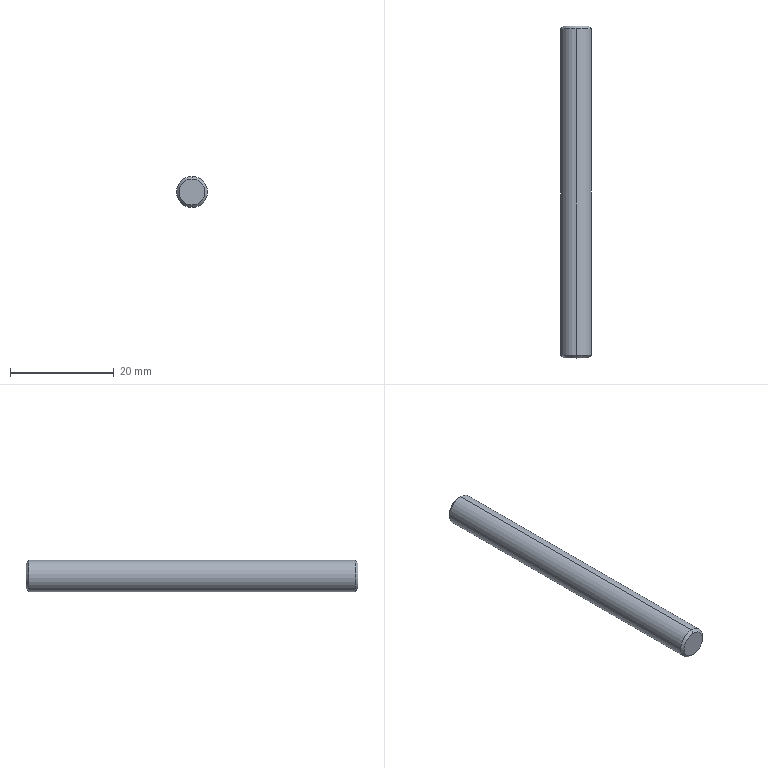Part | NX | features BREP 1 | 1 solid | 8 faces | box 6 x 64 x 6 mm | volume 1805 mm3 | cone 4 | cylinder 2 | plane 2 | commonest cylinder face diameters 6 x2
STEP:
#1=CARTESIAN_POINT('',(0.,64.,2.5));
#2=VERTEX_POINT('',#1);
#3=CARTESIAN_POINT('',(0.,64.,-2.5));
#4=VERTEX_POINT('',#3);
#5=CARTESIAN_POINT('',(0.,64.,0.));
#6=DIRECTION('',(0.,1.,0.));
#7=DIRECTION('',(0.,0.,1.));
#8=AXIS2_PLACEMENT_3D('',#5,#6,#7);
#9=CIRCLE('',#8,2.5);
#10=EDGE_CURVE('',#2,#4,#9,.T.);
#11=ORIENTED_EDGE('',*,*,#10,.F.);
#12=CARTESIAN_POINT('',(0.,63.5,3.));
#13=VERTEX_POINT('',#12);
#14=CARTESIAN_POINT('',(0.,64.,2.5));
#15=DIRECTION('',(0.,-0.7071,0.7071));
#16=VECTOR('',#15,1000.);
#17=LINE('',#14,#16);
#18=EDGE_CURVE('',#13,#2,#17,.F.);
#19=ORIENTED_EDGE('',*,*,#18,.F.);
#20=CARTESIAN_POINT('',(0.,63.5,-3.));
#21=VERTEX_POINT('',#20);
#22=CARTESIAN_POINT('',(0.,63.5,0.));
#23=DIRECTION('',(0.,-1.,0.));
#24=DIRECTION('',(0.,0.,1.));
#25=AXIS2_PLACEMENT_3D('',#22,#23,#24);
#26=CIRCLE('',#25,3.);
#27=EDGE_CURVE('',#21,#13,#26,.T.);
#28=ORIENTED_EDGE('',*,*,#27,.F.);
#29=CARTESIAN_POINT('',(0.,64.,-2.5));
#30=DIRECTION('',(0.,-0.7071,-0.7071));
#31=VECTOR('',#30,1000.);
#32=LINE('',#29,#31);
#33=EDGE_CURVE('',#21,#4,#32,.F.);
#34=ORIENTED_EDGE('',*,*,#33,.T.);
#35=EDGE_LOOP('',(#11,#19,#28,#34));
#36=FACE_BOUND('',#35,.T.);
#37=CARTESIAN_POINT('',(0.,64.,0.));
#38=DIRECTION('',(0.,-1.,0.));
#39=DIRECTION('',(0.,0.,1.));
#40=AXIS2_PLACEMENT_3D('',#37,#38,#39);
#41=CONICAL_SURFACE('',#40,2.5,0.7854);
#42=ADVANCED_FACE('',(#36),#41,.T.);
#43=CARTESIAN_POINT('',(0.,0.,-2.5));
#44=VERTEX_POINT('',#43);
#45=CARTESIAN_POINT('',(0.,0.,2.5));
#46=VERTEX_POINT('',#45);
#47=CARTESIAN_POINT('',(0.,0.,0.));
#48=DIRECTION('',(0.,-1.,0.));
#49=DIRECTION('',(0.,0.,1.));
#50=AXIS2_PLACEMENT_3D('',#47,#48,#49);
#51=CIRCLE('',#50,2.5);
#52=EDGE_CURVE('',#44,#46,#51,.T.);
#53=ORIENTED_EDGE('',*,*,#52,.F.);
#54=CARTESIAN_POINT('',(0.,0.5,-3.));
#55=VERTEX_POINT('',#54);
#56=CARTESIAN_POINT('',(0.,0.5,-3.));
#57=DIRECTION('',(0.,0.7071,-0.7071));
#58=VECTOR('',#57,1000.);
#59=LINE('',#56,#58);
#60=EDGE_CURVE('',#44,#55,#59,.T.);
#61=ORIENTED_EDGE('',*,*,#60,.T.);
#62=CARTESIAN_POINT('',(0.,0.5,3.));
#63=VERTEX_POINT('',#62);
#64=CARTESIAN_POINT('',(0.,0.5,0.));
#65=DIRECTION('',(0.,1.,0.));
#66=DIRECTION('',(0.,0.,1.));
#67=AXIS2_PLACEMENT_3D('',#64,#65,#66);
#68=CIRCLE('',#67,3.);
#69=EDGE_CURVE('',#63,#55,#68,.T.);
#70=ORIENTED_EDGE('',*,*,#69,.F.);
#71=CARTESIAN_POINT('',(0.,0.5,3.));
#72=DIRECTION('',(0.,0.7071,0.7071));
#73=VECTOR('',#72,1000.);
#74=LINE('',#71,#73);
#75=EDGE_CURVE('',#46,#63,#74,.T.);
#76=ORIENTED_EDGE('',*,*,#75,.F.);
#77=EDGE_LOOP('',(#53,#61,#70,#76));
#78=FACE_BOUND('',#77,.T.);
#79=CARTESIAN_POINT('',(0.,0.5,0.));
#80=DIRECTION('',(0.,1.,0.));
#81=DIRECTION('',(0.,0.,-1.));
#82=AXIS2_PLACEMENT_3D('',#79,#80,#81);
#83=CONICAL_SURFACE('',#82,3.,0.7854);
#84=ADVANCED_FACE('',(#78),#83,.T.);
#85=ORIENTED_EDGE('',*,*,#27,.T.);
#86=CARTESIAN_POINT('',(0.,64.,3.));
#87=DIRECTION('',(0.,-1.,0.));
#88=VECTOR('',#87,1000.);
#89=LINE('',#86,#88);
#90=EDGE_CURVE('',#63,#13,#89,.F.);
#91=ORIENTED_EDGE('',*,*,#90,.F.);
#92=ORIENTED_EDGE('',*,*,#69,.T.);
#93=CARTESIAN_POINT('',(0.,64.,-3.));
#94=DIRECTION('',(0.,-1.,0.));
#95=VECTOR('',#94,1000.);
#96=LINE('',#93,#95);
#97=EDGE_CURVE('',#55,#21,#96,.F.);
#98=ORIENTED_EDGE('',*,*,#97,.T.);
#99=EDGE_LOOP('',(#85,#91,#92,#98));
#100=FACE_BOUND('',#99,.T.);
#101=CARTESIAN_POINT('',(0.,64.,0.));
#102=DIRECTION('',(0.,-1.,0.));
#103=DIRECTION('',(0.,0.,1.));
#104=AXIS2_PLACEMENT_3D('',#101,#102,#103);
#105=CYLINDRICAL_SURFACE('',#104,3.);
#106=ADVANCED_FACE('',(#100),#105,.T.);
#107=ORIENTED_EDGE('',*,*,#90,.T.);
#108=CARTESIAN_POINT('',(0.,63.5,0.));
#109=DIRECTION('',(0.,-1.,0.));
#110=DIRECTION('',(0.,0.,1.));
#111=AXIS2_PLACEMENT_3D('',#108,#109,#110);
#112=CIRCLE('',#111,3.);
#113=EDGE_CURVE('',#13,#21,#112,.T.);
#114=ORIENTED_EDGE('',*,*,#113,.T.);
#115=ORIENTED_EDGE('',*,*,#97,.F.);
#116=CARTESIAN_POINT('',(0.,0.5,0.));
#117=DIRECTION('',(0.,1.,0.));
#118=DIRECTION('',(0.,0.,1.));
#119=AXIS2_PLACEMENT_3D('',#116,#117,#118);
#120=CIRCLE('',#119,3.);
#121=EDGE_CURVE('',#55,#63,#120,.T.);
#122=ORIENTED_EDGE('',*,*,#121,.T.);
#123=EDGE_LOOP('',(#107,#114,#115,#122));
#124=FACE_BOUND('',#123,.T.);
#125=CARTESIAN_POINT('',(0.,64.,0.));
#126=DIRECTION('',(0.,-1.,0.));
#127=DIRECTION('',(0.,0.,1.));
#128=AXIS2_PLACEMENT_3D('',#125,#126,#127);
#129=CYLINDRICAL_SURFACE('',#128,3.);
#130=ADVANCED_FACE('',(#124),#129,.T.);
#131=CARTESIAN_POINT('',(0.,64.,0.));
#132=DIRECTION('',(0.,1.,0.));
#133=DIRECTION('',(0.,0.,1.));
#134=AXIS2_PLACEMENT_3D('',#131,#132,#133);
#135=CIRCLE('',#134,2.5);
#136=EDGE_CURVE('',#4,#2,#135,.T.);
#137=ORIENTED_EDGE('',*,*,#136,.T.);
#138=ORIENTED_EDGE('',*,*,#10,.T.);
#139=EDGE_LOOP('',(#137,#138));
#140=FACE_BOUND('',#139,.T.);
#141=CARTESIAN_POINT('',(0.,64.,0.));
#142=DIRECTION('',(0.,1.,0.));
#143=DIRECTION('',(0.,0.,1.));
#144=AXIS2_PLACEMENT_3D('',#141,#142,#143);
#145=PLANE('',#144);
#146=ADVANCED_FACE('',(#140),#145,.T.);
#147=CARTESIAN_POINT('',(0.,0.,0.));
#148=DIRECTION('',(0.,-1.,0.));
#149=DIRECTION('',(0.,0.,1.));
#150=AXIS2_PLACEMENT_3D('',#147,#148,#149);
#151=CIRCLE('',#150,2.5);
#152=EDGE_CURVE('',#46,#44,#151,.T.);
#153=ORIENTED_EDGE('',*,*,#152,.T.);
#154=ORIENTED_EDGE('',*,*,#52,.T.);
#155=EDGE_LOOP('',(#153,#154));
#156=FACE_BOUND('',#155,.T.);
#157=CARTESIAN_POINT('',(0.,0.,0.));
#158=DIRECTION('',(0.,1.,0.));
#159=DIRECTION('',(0.,0.,1.));
#160=AXIS2_PLACEMENT_3D('',#157,#158,#159);
#161=PLANE('',#160);
#162=ADVANCED_FACE('',(#156),#161,.F.);
#163=ORIENTED_EDGE('',*,*,#60,.F.);
#164=ORIENTED_EDGE('',*,*,#152,.F.);
#165=ORIENTED_EDGE('',*,*,#75,.T.);
#166=ORIENTED_EDGE('',*,*,#121,.F.);
#167=EDGE_LOOP('',(#163,#164,#165,#166));
#168=FACE_BOUND('',#167,.T.);
#169=CARTESIAN_POINT('',(0.,0.5,0.));
#170=DIRECTION('',(0.,1.,0.));
#171=DIRECTION('',(0.,0.,-1.));
#172=AXIS2_PLACEMENT_3D('',#169,#170,#171);
#173=CONICAL_SURFACE('',#172,3.,0.7854);
#174=ADVANCED_FACE('',(#168),#173,.T.);
#175=ORIENTED_EDGE('',*,*,#18,.T.);
#176=ORIENTED_EDGE('',*,*,#136,.F.);
#177=ORIENTED_EDGE('',*,*,#33,.F.);
#178=ORIENTED_EDGE('',*,*,#113,.F.);
#179=EDGE_LOOP('',(#175,#176,#177,#178));
#180=FACE_BOUND('',#179,.T.);
#181=CARTESIAN_POINT('',(0.,64.,0.));
#182=DIRECTION('',(0.,-1.,0.));
#183=DIRECTION('',(0.,0.,1.));
#184=AXIS2_PLACEMENT_3D('',#181,#182,#183);
#185=CONICAL_SURFACE('',#184,2.5,0.7854);
#186=ADVANCED_FACE('',(#180),#185,.T.);
#187=CLOSED_SHELL('',(#42,#84,#106,#130,#146,#162,#174,#186));
#188=MANIFOLD_SOLID_BREP('',#187);
#189=(LENGTH_UNIT()NAMED_UNIT(*)SI_UNIT(.MILLI.,.METRE.));
#190=UNCERTAINTY_MEASURE_WITH_UNIT(LENGTH_MEASURE(0.00001),#189,'','');
#191=(NAMED_UNIT(*)PLANE_ANGLE_UNIT()SI_UNIT($,.RADIAN.));
#192=(NAMED_UNIT(*)SI_UNIT($,.STERADIAN.)SOLID_ANGLE_UNIT());
#193=(GEOMETRIC_REPRESENTATION_CONTEXT(3)GLOBAL_UNCERTAINTY_ASSIGNED_CONTEXT((#190))GLOBAL_UNIT_ASSIGNED_CONTEXT((#189,#191,#192))REPRESENTATION_CONTEXT('',''));
#194=ADVANCED_BREP_SHAPE_REPRESENTATION('',(#188),#193);